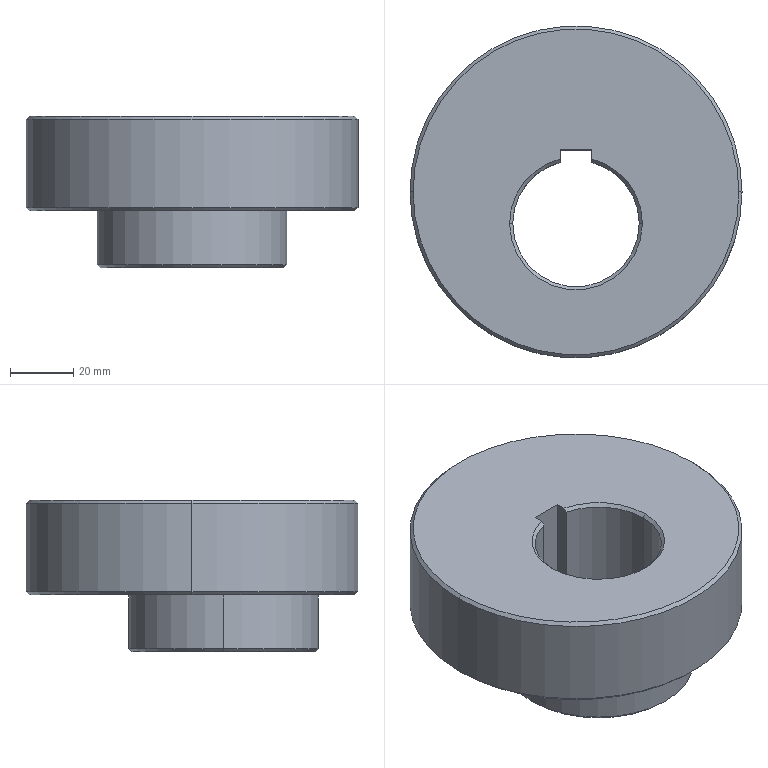Part | SolidWorks | features Boss 1, Chamfer 1, Cut 1, Extrusion 1 | 1 solid | 25 faces | box 105 x 105 x 48 mm | volume 248122 mm3 | cone 12 | cylinder 7 | plane 6 | commonest cylinder face diameters 40 x3 60 x2 105 x2
STEP:
#1=CARTESIAN_POINT('',(20.,0.,-17.));
#2=VERTEX_POINT('',#1);
#3=CARTESIAN_POINT('',(-20.,0.,-17.));
#4=VERTEX_POINT('',#3);
#5=CARTESIAN_POINT('',(0.,0.,-17.));
#6=DIRECTION('',(0.,0.,-1.));
#7=DIRECTION('',(1.,0.,0.));
#8=AXIS2_PLACEMENT_3D('',#5,#6,#7);
#9=CIRCLE('',#8,20.);
#10=EDGE_CURVE('',#2,#4,#9,.T.);
#11=ORIENTED_EDGE('',*,*,#10,.F.);
#12=CARTESIAN_POINT('',(21.,0.,-18.));
#13=VERTEX_POINT('',#12);
#14=CARTESIAN_POINT('',(21.,0.,-18.));
#15=DIRECTION('',(0.7071,0.,-0.7071));
#16=VECTOR('',#15,1000.);
#17=LINE('',#14,#16);
#18=EDGE_CURVE('',#2,#13,#17,.T.);
#19=ORIENTED_EDGE('',*,*,#18,.T.);
#20=CARTESIAN_POINT('',(-21.,0.,-18.));
#21=VERTEX_POINT('',#20);
#22=CARTESIAN_POINT('',(0.,0.,-18.));
#23=DIRECTION('',(0.,0.,1.));
#24=DIRECTION('',(1.,0.,0.));
#25=AXIS2_PLACEMENT_3D('',#22,#23,#24);
#26=CIRCLE('',#25,21.);
#27=EDGE_CURVE('',#21,#13,#26,.T.);
#28=ORIENTED_EDGE('',*,*,#27,.F.);
#29=CARTESIAN_POINT('',(-21.,0.,-18.));
#30=DIRECTION('',(-0.7071,0.,-0.7071));
#31=VECTOR('',#30,1000.);
#32=LINE('',#29,#31);
#33=EDGE_CURVE('',#4,#21,#32,.T.);
#34=ORIENTED_EDGE('',*,*,#33,.F.);
#35=EDGE_LOOP('',(#11,#19,#28,#34));
#36=FACE_OUTER_BOUND('',#35,.T.);
#37=CARTESIAN_POINT('',(0.,0.,-18.));
#38=DIRECTION('',(0.,0.,-1.));
#39=DIRECTION('',(-1.,0.,0.));
#40=AXIS2_PLACEMENT_3D('',#37,#38,#39);
#41=CONICAL_SURFACE('',#40,21.,0.7854);
#42=ADVANCED_FACE('',(#36),#41,.F.);
#43=CARTESIAN_POINT('',(-5.,19.365,-17.));
#44=VERTEX_POINT('',#43);
#45=CARTESIAN_POINT('',(0.,0.,-17.));
#46=DIRECTION('',(0.,0.,-1.));
#47=DIRECTION('',(1.,0.,0.));
#48=AXIS2_PLACEMENT_3D('',#45,#46,#47);
#49=CIRCLE('',#48,20.);
#50=EDGE_CURVE('',#4,#44,#49,.T.);
#51=ORIENTED_EDGE('',*,*,#50,.F.);
#52=ORIENTED_EDGE('',*,*,#33,.T.);
#53=CARTESIAN_POINT('',(-5.,20.396,-18.));
#54=VERTEX_POINT('',#53);
#55=CARTESIAN_POINT('',(0.,0.,-18.));
#56=DIRECTION('',(0.,0.,1.));
#57=DIRECTION('',(1.,0.,0.));
#58=AXIS2_PLACEMENT_3D('',#55,#56,#57);
#59=CIRCLE('',#58,21.);
#60=EDGE_CURVE('',#54,#21,#59,.T.);
#61=ORIENTED_EDGE('',*,*,#60,.F.);
#62=CARTESIAN_POINT('',(-5.,19.365,-17.));
#63=CARTESIAN_POINT('',(-5.,19.709,-17.333));
#64=CARTESIAN_POINT('',(-5.,20.053,-17.666));
#65=CARTESIAN_POINT('',(-5.,20.396,-18.));
#66=B_SPLINE_CURVE_WITH_KNOTS('',3,(#62,#63,#64,#65),.UNSPECIFIED.,.F.,.F.,(4,4),(0.,0.001436),.UNSPECIFIED.);
#67=EDGE_CURVE('',#44,#54,#66,.T.);
#68=ORIENTED_EDGE('',*,*,#67,.F.);
#69=EDGE_LOOP('',(#51,#52,#61,#68));
#70=FACE_OUTER_BOUND('',#69,.T.);
#71=CARTESIAN_POINT('',(0.,0.,-18.));
#72=DIRECTION('',(0.,0.,-1.));
#73=DIRECTION('',(-1.,0.,0.));
#74=AXIS2_PLACEMENT_3D('',#71,#72,#73);
#75=CONICAL_SURFACE('',#74,21.,0.7854);
#76=ADVANCED_FACE('',(#70),#75,.F.);
#77=CARTESIAN_POINT('',(-20.,0.,29.));
#78=VERTEX_POINT('',#77);
#79=CARTESIAN_POINT('',(20.,0.,29.));
#80=VERTEX_POINT('',#79);
#81=CARTESIAN_POINT('',(0.,0.,29.));
#82=DIRECTION('',(0.,0.,1.));
#83=DIRECTION('',(1.,0.,0.));
#84=AXIS2_PLACEMENT_3D('',#81,#82,#83);
#85=CIRCLE('',#84,20.);
#86=EDGE_CURVE('',#78,#80,#85,.T.);
#87=ORIENTED_EDGE('',*,*,#86,.F.);
#88=CARTESIAN_POINT('',(-21.,0.,30.));
#89=VERTEX_POINT('',#88);
#90=CARTESIAN_POINT('',(-20.,0.,29.));
#91=DIRECTION('',(-0.7071,0.,0.7071));
#92=VECTOR('',#91,1000.);
#93=LINE('',#90,#92);
#94=EDGE_CURVE('',#78,#89,#93,.T.);
#95=ORIENTED_EDGE('',*,*,#94,.T.);
#96=CARTESIAN_POINT('',(21.,0.,30.));
#97=VERTEX_POINT('',#96);
#98=CARTESIAN_POINT('',(0.,0.,30.));
#99=DIRECTION('',(0.,0.,-1.));
#100=DIRECTION('',(1.,0.,0.));
#101=AXIS2_PLACEMENT_3D('',#98,#99,#100);
#102=CIRCLE('',#101,21.);
#103=EDGE_CURVE('',#97,#89,#102,.T.);
#104=ORIENTED_EDGE('',*,*,#103,.F.);
#105=CARTESIAN_POINT('',(20.,0.,29.));
#106=DIRECTION('',(0.7071,0.,0.7071));
#107=VECTOR('',#106,1000.);
#108=LINE('',#105,#107);
#109=EDGE_CURVE('',#80,#97,#108,.T.);
#110=ORIENTED_EDGE('',*,*,#109,.F.);
#111=EDGE_LOOP('',(#87,#95,#104,#110));
#112=FACE_OUTER_BOUND('',#111,.T.);
#113=CARTESIAN_POINT('',(0.,0.,29.));
#114=DIRECTION('',(0.,0.,1.));
#115=DIRECTION('',(1.,0.,0.));
#116=AXIS2_PLACEMENT_3D('',#113,#114,#115);
#117=CONICAL_SURFACE('',#116,20.,0.7854);
#118=ADVANCED_FACE('',(#112),#117,.F.);
#119=CARTESIAN_POINT('',(5.,19.365,29.));
#120=VERTEX_POINT('',#119);
#121=CARTESIAN_POINT('',(0.,0.,29.));
#122=DIRECTION('',(0.,0.,1.));
#123=DIRECTION('',(1.,0.,0.));
#124=AXIS2_PLACEMENT_3D('',#121,#122,#123);
#125=CIRCLE('',#124,20.);
#126=EDGE_CURVE('',#80,#120,#125,.T.);
#127=ORIENTED_EDGE('',*,*,#126,.F.);
#128=ORIENTED_EDGE('',*,*,#109,.T.);
#129=CARTESIAN_POINT('',(5.,20.396,30.));
#130=VERTEX_POINT('',#129);
#131=CARTESIAN_POINT('',(0.,0.,30.));
#132=DIRECTION('',(0.,0.,-1.));
#133=DIRECTION('',(1.,0.,0.));
#134=AXIS2_PLACEMENT_3D('',#131,#132,#133);
#135=CIRCLE('',#134,21.);
#136=EDGE_CURVE('',#130,#97,#135,.T.);
#137=ORIENTED_EDGE('',*,*,#136,.F.);
#138=CARTESIAN_POINT('',(5.,19.365,29.));
#139=CARTESIAN_POINT('',(5.,19.709,29.333));
#140=CARTESIAN_POINT('',(5.,20.053,29.666));
#141=CARTESIAN_POINT('',(5.,20.396,30.));
#142=B_SPLINE_CURVE_WITH_KNOTS('',3,(#138,#139,#140,#141),.UNSPECIFIED.,.F.,.F.,(4,4),(0.,0.001436),.UNSPECIFIED.);
#143=EDGE_CURVE('',#120,#130,#142,.T.);
#144=ORIENTED_EDGE('',*,*,#143,.F.);
#145=EDGE_LOOP('',(#127,#128,#137,#144));
#146=FACE_OUTER_BOUND('',#145,.T.);
#147=CARTESIAN_POINT('',(0.,0.,29.));
#148=DIRECTION('',(0.,0.,1.));
#149=DIRECTION('',(1.,0.,0.));
#150=AXIS2_PLACEMENT_3D('',#147,#148,#149);
#151=CONICAL_SURFACE('',#150,20.,0.7854);
#152=ADVANCED_FACE('',(#146),#151,.F.);
#153=CARTESIAN_POINT('',(-29.,0.,-18.));
#154=VERTEX_POINT('',#153);
#155=CARTESIAN_POINT('',(29.,0.,-18.));
#156=VERTEX_POINT('',#155);
#157=CARTESIAN_POINT('',(0.,0.,-18.));
#158=DIRECTION('',(0.,0.,-1.));
#159=DIRECTION('',(1.,0.,0.));
#160=AXIS2_PLACEMENT_3D('',#157,#158,#159);
#161=CIRCLE('',#160,29.);
#162=EDGE_CURVE('',#154,#156,#161,.T.);
#163=ORIENTED_EDGE('',*,*,#162,.F.);
#164=CARTESIAN_POINT('',(-30.,0.,-17.));
#165=VERTEX_POINT('',#164);
#166=CARTESIAN_POINT('',(-30.,0.,-17.));
#167=DIRECTION('',(-0.7071,0.,0.7071));
#168=VECTOR('',#167,1000.);
#169=LINE('',#166,#168);
#170=EDGE_CURVE('',#154,#165,#169,.T.);
#171=ORIENTED_EDGE('',*,*,#170,.T.);
#172=CARTESIAN_POINT('',(30.,0.,-17.));
#173=VERTEX_POINT('',#172);
#174=CARTESIAN_POINT('',(0.,0.,-17.));
#175=DIRECTION('',(0.,0.,1.));
#176=DIRECTION('',(1.,0.,0.));
#177=AXIS2_PLACEMENT_3D('',#174,#175,#176);
#178=CIRCLE('',#177,30.);
#179=EDGE_CURVE('',#173,#165,#178,.T.);
#180=ORIENTED_EDGE('',*,*,#179,.F.);
#181=CARTESIAN_POINT('',(30.,0.,-17.));
#182=DIRECTION('',(0.7071,0.,0.7071));
#183=VECTOR('',#182,1000.);
#184=LINE('',#181,#183);
#185=EDGE_CURVE('',#156,#173,#184,.T.);
#186=ORIENTED_EDGE('',*,*,#185,.F.);
#187=EDGE_LOOP('',(#163,#171,#180,#186));
#188=FACE_OUTER_BOUND('',#187,.T.);
#189=CARTESIAN_POINT('',(0.,0.,-17.));
#190=DIRECTION('',(0.,0.,1.));
#191=DIRECTION('',(1.,0.,0.));
#192=AXIS2_PLACEMENT_3D('',#189,#190,#191);
#193=CONICAL_SURFACE('',#192,30.,0.7854);
#194=ADVANCED_FACE('',(#188),#193,.T.);
#195=CARTESIAN_POINT('',(-51.5,10.,0.));
#196=VERTEX_POINT('',#195);
#197=CARTESIAN_POINT('',(51.5,10.,0.));
#198=VERTEX_POINT('',#197);
#199=CARTESIAN_POINT('',(0.,10.,0.));
#200=DIRECTION('',(0.,0.,-1.));
#201=DIRECTION('',(1.,0.,0.));
#202=AXIS2_PLACEMENT_3D('',#199,#200,#201);
#203=CIRCLE('',#202,51.5);
#204=EDGE_CURVE('',#196,#198,#203,.T.);
#205=ORIENTED_EDGE('',*,*,#204,.F.);
#206=CARTESIAN_POINT('',(-52.5,10.,1.));
#207=VERTEX_POINT('',#206);
#208=CARTESIAN_POINT('',(-52.5,10.,1.));
#209=DIRECTION('',(-0.7071,0.,0.7071));
#210=VECTOR('',#209,1000.);
#211=LINE('',#208,#210);
#212=EDGE_CURVE('',#196,#207,#211,.T.);
#213=ORIENTED_EDGE('',*,*,#212,.T.);
#214=CARTESIAN_POINT('',(52.5,10.,1.));
#215=VERTEX_POINT('',#214);
#216=CARTESIAN_POINT('',(0.,10.,1.));
#217=DIRECTION('',(0.,0.,1.));
#218=DIRECTION('',(1.,0.,0.));
#219=AXIS2_PLACEMENT_3D('',#216,#217,#218);
#220=CIRCLE('',#219,52.5);
#221=EDGE_CURVE('',#215,#207,#220,.T.);
#222=ORIENTED_EDGE('',*,*,#221,.F.);
#223=CARTESIAN_POINT('',(52.5,10.,1.));
#224=DIRECTION('',(0.7071,0.,0.7071));
#225=VECTOR('',#224,1000.);
#226=LINE('',#223,#225);
#227=EDGE_CURVE('',#198,#215,#226,.T.);
#228=ORIENTED_EDGE('',*,*,#227,.F.);
#229=EDGE_LOOP('',(#205,#213,#222,#228));
#230=FACE_OUTER_BOUND('',#229,.T.);
#231=CARTESIAN_POINT('',(0.,10.,1.));
#232=DIRECTION('',(0.,0.,1.));
#233=DIRECTION('',(1.,0.,0.));
#234=AXIS2_PLACEMENT_3D('',#231,#232,#233);
#235=CONICAL_SURFACE('',#234,52.5,0.7854);
#236=ADVANCED_FACE('',(#230),#235,.T.);
#237=CARTESIAN_POINT('',(51.5,10.,30.));
#238=VERTEX_POINT('',#237);
#239=CARTESIAN_POINT('',(-51.5,10.,30.));
#240=VERTEX_POINT('',#239);
#241=CARTESIAN_POINT('',(0.,10.,30.));
#242=DIRECTION('',(0.,0.,1.));
#243=DIRECTION('',(1.,0.,0.));
#244=AXIS2_PLACEMENT_3D('',#241,#242,#243);
#245=CIRCLE('',#244,51.5);
#246=EDGE_CURVE('',#238,#240,#245,.T.);
#247=ORIENTED_EDGE('',*,*,#246,.F.);
#248=CARTESIAN_POINT('',(52.5,10.,29.));
#249=VERTEX_POINT('',#248);
#250=CARTESIAN_POINT('',(51.5,10.,30.));
#251=DIRECTION('',(0.7071,0.,-0.7071));
#252=VECTOR('',#251,1000.);
#253=LINE('',#250,#252);
#254=EDGE_CURVE('',#238,#249,#253,.T.);
#255=ORIENTED_EDGE('',*,*,#254,.T.);
#256=CARTESIAN_POINT('',(-52.5,10.,29.));
#257=VERTEX_POINT('',#256);
#258=CARTESIAN_POINT('',(0.,10.,29.));
#259=DIRECTION('',(0.,0.,-1.));
#260=DIRECTION('',(1.,0.,0.));
#261=AXIS2_PLACEMENT_3D('',#258,#259,#260);
#262=CIRCLE('',#261,52.5);
#263=EDGE_CURVE('',#257,#249,#262,.T.);
#264=ORIENTED_EDGE('',*,*,#263,.F.);
#265=CARTESIAN_POINT('',(-51.5,10.,30.));
#266=DIRECTION('',(-0.7071,0.,-0.7071));
#267=VECTOR('',#266,1000.);
#268=LINE('',#265,#267);
#269=EDGE_CURVE('',#240,#257,#268,.T.);
#270=ORIENTED_EDGE('',*,*,#269,.F.);
#271=EDGE_LOOP('',(#247,#255,#264,#270));
#272=FACE_OUTER_BOUND('',#271,.T.);
#273=CARTESIAN_POINT('',(0.,10.,30.));
#274=DIRECTION('',(0.,0.,-1.));
#275=DIRECTION('',(-1.,0.,0.));
#276=AXIS2_PLACEMENT_3D('',#273,#274,#275);
#277=CONICAL_SURFACE('',#276,51.5,0.7854);
#278=ADVANCED_FACE('',(#272),#277,.T.);
#279=ORIENTED_EDGE('',*,*,#10,.T.);
#280=CARTESIAN_POINT('',(-20.,0.,-18.));
#281=DIRECTION('',(0.,0.,1.));
#282=VECTOR('',#281,1000.);
#283=LINE('',#280,#282);
#284=EDGE_CURVE('',#4,#78,#283,.T.);
#285=ORIENTED_EDGE('',*,*,#284,.T.);
#286=ORIENTED_EDGE('',*,*,#86,.T.);
#287=CARTESIAN_POINT('',(20.,0.,-18.));
#288=DIRECTION('',(0.,0.,1.));
#289=VECTOR('',#288,1000.);
#290=LINE('',#287,#289);
#291=EDGE_CURVE('',#2,#80,#290,.T.);
#292=ORIENTED_EDGE('',*,*,#291,.F.);
#293=EDGE_LOOP('',(#279,#285,#286,#292));
#294=FACE_OUTER_BOUND('',#293,.T.);
#295=CARTESIAN_POINT('',(0.,0.,-18.));
#296=DIRECTION('',(0.,0.,1.));
#297=DIRECTION('',(1.,0.,0.));
#298=AXIS2_PLACEMENT_3D('',#295,#296,#297);
#299=CYLINDRICAL_SURFACE('',#298,20.);
#300=ADVANCED_FACE('',(#294),#299,.F.);
#301=CARTESIAN_POINT('',(5.,19.365,-17.));
#302=VERTEX_POINT('',#301);
#303=CARTESIAN_POINT('',(0.,0.,-17.));
#304=DIRECTION('',(0.,0.,-1.));
#305=DIRECTION('',(1.,0.,0.));
#306=AXIS2_PLACEMENT_3D('',#303,#304,#305);
#307=CIRCLE('',#306,20.);
#308=EDGE_CURVE('',#302,#2,#307,.T.);
#309=ORIENTED_EDGE('',*,*,#308,.T.);
#310=ORIENTED_EDGE('',*,*,#291,.T.);
#311=ORIENTED_EDGE('',*,*,#126,.T.);
#312=CARTESIAN_POINT('',(5.,19.365,-18.));
#313=DIRECTION('',(0.,0.,1.));
#314=VECTOR('',#313,1000.);
#315=LINE('',#312,#314);
#316=EDGE_CURVE('',#302,#120,#315,.T.);
#317=ORIENTED_EDGE('',*,*,#316,.F.);
#318=EDGE_LOOP('',(#309,#310,#311,#317));
#319=FACE_OUTER_BOUND('',#318,.T.);
#320=CARTESIAN_POINT('',(0.,0.,-18.));
#321=DIRECTION('',(0.,0.,1.));
#322=DIRECTION('',(1.,0.,0.));
#323=AXIS2_PLACEMENT_3D('',#320,#321,#322);
#324=CYLINDRICAL_SURFACE('',#323,20.);
#325=ADVANCED_FACE('',(#319),#324,.F.);
#326=ORIENTED_EDGE('',*,*,#179,.T.);
#327=CARTESIAN_POINT('',(-30.,0.,0.));
#328=VERTEX_POINT('',#327);
#329=CARTESIAN_POINT('',(-30.,0.,-18.));
#330=DIRECTION('',(0.,0.,1.));
#331=VECTOR('',#330,1000.);
#332=LINE('',#329,#331);
#333=EDGE_CURVE('',#165,#328,#332,.T.);
#334=ORIENTED_EDGE('',*,*,#333,.T.);
#335=CARTESIAN_POINT('',(30.,0.,0.));
#336=VERTEX_POINT('',#335);
#337=CARTESIAN_POINT('',(0.,0.,0.));
#338=DIRECTION('',(0.,0.,1.));
#339=DIRECTION('',(1.,0.,0.));
#340=AXIS2_PLACEMENT_3D('',#337,#338,#339);
#341=CIRCLE('',#340,30.);
#342=EDGE_CURVE('',#336,#328,#341,.T.);
#343=ORIENTED_EDGE('',*,*,#342,.F.);
#344=CARTESIAN_POINT('',(30.,0.,-18.));
#345=DIRECTION('',(0.,0.,1.));
#346=VECTOR('',#345,1000.);
#347=LINE('',#344,#346);
#348=EDGE_CURVE('',#173,#336,#347,.T.);
#349=ORIENTED_EDGE('',*,*,#348,.F.);
#350=EDGE_LOOP('',(#326,#334,#343,#349));
#351=FACE_OUTER_BOUND('',#350,.T.);
#352=CARTESIAN_POINT('',(0.,0.,-18.));
#353=DIRECTION('',(0.,0.,1.));
#354=DIRECTION('',(1.,0.,0.));
#355=AXIS2_PLACEMENT_3D('',#352,#353,#354);
#356=CYLINDRICAL_SURFACE('',#355,30.);
#357=ADVANCED_FACE('',(#351),#356,.T.);
#358=ORIENTED_EDGE('',*,*,#263,.T.);
#359=CARTESIAN_POINT('',(52.5,10.,30.));
#360=DIRECTION('',(0.,0.,-1.));
#361=VECTOR('',#360,1000.);
#362=LINE('',#359,#361);
#363=EDGE_CURVE('',#249,#215,#362,.T.);
#364=ORIENTED_EDGE('',*,*,#363,.T.);
#365=ORIENTED_EDGE('',*,*,#221,.T.);
#366=CARTESIAN_POINT('',(-52.5,10.,30.));
#367=DIRECTION('',(0.,0.,-1.));
#368=VECTOR('',#367,1000.);
#369=LINE('',#366,#368);
#370=EDGE_CURVE('',#257,#207,#369,.T.);
#371=ORIENTED_EDGE('',*,*,#370,.F.);
#372=EDGE_LOOP('',(#358,#364,#365,#371));
#373=FACE_OUTER_BOUND('',#372,.T.);
#374=CARTESIAN_POINT('',(0.,10.,30.));
#375=DIRECTION('',(0.,0.,-1.));
#376=DIRECTION('',(-1.,0.,0.));
#377=AXIS2_PLACEMENT_3D('',#374,#375,#376);
#378=CYLINDRICAL_SURFACE('',#377,52.5);
#379=ADVANCED_FACE('',(#373),#378,.T.);
#380=CARTESIAN_POINT('',(0.,10.,30.));
#381=DIRECTION('',(0.,0.,1.));
#382=DIRECTION('',(1.,0.,0.));
#383=AXIS2_PLACEMENT_3D('',#380,#381,#382);
#384=CIRCLE('',#383,51.5);
#385=EDGE_CURVE('',#240,#238,#384,.T.);
#386=ORIENTED_EDGE('',*,*,#385,.T.);
#387=ORIENTED_EDGE('',*,*,#246,.T.);
#388=EDGE_LOOP('',(#386,#387));
#389=FACE_OUTER_BOUND('',#388,.T.);
#390=CARTESIAN_POINT('',(5.,23.3,30.));
#391=VERTEX_POINT('',#390);
#392=CARTESIAN_POINT('',(5.,19.365,30.));
#393=DIRECTION('',(0.,1.,0.));
#394=VECTOR('',#393,1000.);
#395=LINE('',#392,#394);
#396=EDGE_CURVE('',#130,#391,#395,.T.);
#397=ORIENTED_EDGE('',*,*,#396,.F.);
#398=ORIENTED_EDGE('',*,*,#136,.T.);
#399=ORIENTED_EDGE('',*,*,#103,.T.);
#400=CARTESIAN_POINT('',(-5.,20.396,30.));
#401=VERTEX_POINT('',#400);
#402=CARTESIAN_POINT('',(0.,0.,30.));
#403=DIRECTION('',(0.,0.,-1.));
#404=DIRECTION('',(1.,0.,0.));
#405=AXIS2_PLACEMENT_3D('',#402,#403,#404);
#406=CIRCLE('',#405,21.);
#407=EDGE_CURVE('',#89,#401,#406,.T.);
#408=ORIENTED_EDGE('',*,*,#407,.T.);
#409=CARTESIAN_POINT('',(-5.,23.3,30.));
#410=VERTEX_POINT('',#409);
#411=CARTESIAN_POINT('',(-5.,23.3,30.));
#412=DIRECTION('',(0.,-1.,0.));
#413=VECTOR('',#412,1000.);
#414=LINE('',#411,#413);
#415=EDGE_CURVE('',#410,#401,#414,.T.);
#416=ORIENTED_EDGE('',*,*,#415,.F.);
#417=CARTESIAN_POINT('',(5.,23.3,30.));
#418=DIRECTION('',(-1.,0.,0.));
#419=VECTOR('',#418,1000.);
#420=LINE('',#417,#419);
#421=EDGE_CURVE('',#391,#410,#420,.T.);
#422=ORIENTED_EDGE('',*,*,#421,.F.);
#423=EDGE_LOOP('',(#397,#398,#399,#408,#416,#422));
#424=FACE_BOUND('',#423,.T.);
#425=CARTESIAN_POINT('',(0.,10.,30.));
#426=DIRECTION('',(0.,0.,1.));
#427=DIRECTION('',(1.,0.,0.));
#428=AXIS2_PLACEMENT_3D('',#425,#426,#427);
#429=PLANE('',#428);
#430=ADVANCED_FACE('',(#389,#424),#429,.T.);
#431=ORIENTED_EDGE('',*,*,#363,.F.);
#432=CARTESIAN_POINT('',(0.,10.,29.));
#433=DIRECTION('',(0.,0.,-1.));
#434=DIRECTION('',(1.,0.,0.));
#435=AXIS2_PLACEMENT_3D('',#432,#433,#434);
#436=CIRCLE('',#435,52.5);
#437=EDGE_CURVE('',#249,#257,#436,.T.);
#438=ORIENTED_EDGE('',*,*,#437,.T.);
#439=ORIENTED_EDGE('',*,*,#370,.T.);
#440=CARTESIAN_POINT('',(0.,10.,1.));
#441=DIRECTION('',(0.,0.,1.));
#442=DIRECTION('',(1.,0.,0.));
#443=AXIS2_PLACEMENT_3D('',#440,#441,#442);
#444=CIRCLE('',#443,52.5);
#445=EDGE_CURVE('',#207,#215,#444,.T.);
#446=ORIENTED_EDGE('',*,*,#445,.T.);
#447=EDGE_LOOP('',(#431,#438,#439,#446));
#448=FACE_OUTER_BOUND('',#447,.T.);
#449=CARTESIAN_POINT('',(0.,10.,30.));
#450=DIRECTION('',(0.,0.,-1.));
#451=DIRECTION('',(-1.,0.,0.));
#452=AXIS2_PLACEMENT_3D('',#449,#450,#451);
#453=CYLINDRICAL_SURFACE('',#452,52.5);
#454=ADVANCED_FACE('',(#448),#453,.T.);
#455=CARTESIAN_POINT('',(0.,10.,0.));
#456=DIRECTION('',(0.,0.,-1.));
#457=DIRECTION('',(1.,0.,0.));
#458=AXIS2_PLACEMENT_3D('',#455,#456,#457);
#459=CIRCLE('',#458,51.5);
#460=EDGE_CURVE('',#198,#196,#459,.T.);
#461=ORIENTED_EDGE('',*,*,#460,.T.);
#462=ORIENTED_EDGE('',*,*,#204,.T.);
#463=EDGE_LOOP('',(#461,#462));
#464=FACE_OUTER_BOUND('',#463,.T.);
#465=ORIENTED_EDGE('',*,*,#342,.T.);
#466=CARTESIAN_POINT('',(0.,0.,0.));
#467=DIRECTION('',(0.,0.,1.));
#468=DIRECTION('',(1.,0.,0.));
#469=AXIS2_PLACEMENT_3D('',#466,#467,#468);
#470=CIRCLE('',#469,30.);
#471=EDGE_CURVE('',#328,#336,#470,.T.);
#472=ORIENTED_EDGE('',*,*,#471,.T.);
#473=EDGE_LOOP('',(#465,#472));
#474=FACE_BOUND('',#473,.T.);
#475=CARTESIAN_POINT('',(0.,10.,0.));
#476=DIRECTION('',(0.,0.,1.));
#477=DIRECTION('',(1.,0.,0.));
#478=AXIS2_PLACEMENT_3D('',#475,#476,#477);
#479=PLANE('',#478);
#480=ADVANCED_FACE('',(#464,#474),#479,.F.);
#481=ORIENTED_EDGE('',*,*,#333,.F.);
#482=CARTESIAN_POINT('',(0.,0.,-17.));
#483=DIRECTION('',(0.,0.,1.));
#484=DIRECTION('',(1.,0.,0.));
#485=AXIS2_PLACEMENT_3D('',#482,#483,#484);
#486=CIRCLE('',#485,30.);
#487=EDGE_CURVE('',#165,#173,#486,.T.);
#488=ORIENTED_EDGE('',*,*,#487,.T.);
#489=ORIENTED_EDGE('',*,*,#348,.T.);
#490=ORIENTED_EDGE('',*,*,#471,.F.);
#491=EDGE_LOOP('',(#481,#488,#489,#490));
#492=FACE_OUTER_BOUND('',#491,.T.);
#493=CARTESIAN_POINT('',(0.,0.,-18.));
#494=DIRECTION('',(0.,0.,1.));
#495=DIRECTION('',(1.,0.,0.));
#496=AXIS2_PLACEMENT_3D('',#493,#494,#495);
#497=CYLINDRICAL_SURFACE('',#496,30.);
#498=ADVANCED_FACE('',(#492),#497,.T.);
#499=CARTESIAN_POINT('',(0.,0.,-18.));
#500=DIRECTION('',(0.,0.,-1.));
#501=DIRECTION('',(1.,0.,0.));
#502=AXIS2_PLACEMENT_3D('',#499,#500,#501);
#503=CIRCLE('',#502,29.);
#504=EDGE_CURVE('',#156,#154,#503,.T.);
#505=ORIENTED_EDGE('',*,*,#504,.T.);
#506=ORIENTED_EDGE('',*,*,#162,.T.);
#507=EDGE_LOOP('',(#505,#506));
#508=FACE_OUTER_BOUND('',#507,.T.);
#509=CARTESIAN_POINT('',(-5.,23.3,-18.));
#510=VERTEX_POINT('',#509);
#511=CARTESIAN_POINT('',(-5.,23.3,-18.));
#512=DIRECTION('',(0.,-1.,0.));
#513=VECTOR('',#512,1000.);
#514=LINE('',#511,#513);
#515=EDGE_CURVE('',#510,#54,#514,.T.);
#516=ORIENTED_EDGE('',*,*,#515,.T.);
#517=ORIENTED_EDGE('',*,*,#60,.T.);
#518=ORIENTED_EDGE('',*,*,#27,.T.);
#519=CARTESIAN_POINT('',(5.,20.396,-18.));
#520=VERTEX_POINT('',#519);
#521=CARTESIAN_POINT('',(0.,0.,-18.));
#522=DIRECTION('',(0.,0.,1.));
#523=DIRECTION('',(1.,0.,0.));
#524=AXIS2_PLACEMENT_3D('',#521,#522,#523);
#525=CIRCLE('',#524,21.);
#526=EDGE_CURVE('',#13,#520,#525,.T.);
#527=ORIENTED_EDGE('',*,*,#526,.T.);
#528=CARTESIAN_POINT('',(5.,23.3,-18.));
#529=VERTEX_POINT('',#528);
#530=CARTESIAN_POINT('',(5.,19.365,-18.));
#531=DIRECTION('',(0.,1.,0.));
#532=VECTOR('',#531,1000.);
#533=LINE('',#530,#532);
#534=EDGE_CURVE('',#520,#529,#533,.T.);
#535=ORIENTED_EDGE('',*,*,#534,.T.);
#536=CARTESIAN_POINT('',(5.,23.3,-18.));
#537=DIRECTION('',(-1.,0.,0.));
#538=VECTOR('',#537,1000.);
#539=LINE('',#536,#538);
#540=EDGE_CURVE('',#529,#510,#539,.T.);
#541=ORIENTED_EDGE('',*,*,#540,.T.);
#542=EDGE_LOOP('',(#516,#517,#518,#527,#535,#541));
#543=FACE_BOUND('',#542,.T.);
#544=CARTESIAN_POINT('',(0.,0.,-18.));
#545=DIRECTION('',(0.,0.,1.));
#546=DIRECTION('',(1.,0.,0.));
#547=AXIS2_PLACEMENT_3D('',#544,#545,#546);
#548=PLANE('',#547);
#549=ADVANCED_FACE('',(#508,#543),#548,.F.);
#550=ORIENTED_EDGE('',*,*,#415,.T.);
#551=CARTESIAN_POINT('',(-5.,19.365,29.));
#552=VERTEX_POINT('',#551);
#553=CARTESIAN_POINT('',(-5.,20.396,30.));
#554=CARTESIAN_POINT('',(-5.,20.053,29.666));
#555=CARTESIAN_POINT('',(-5.,19.709,29.333));
#556=CARTESIAN_POINT('',(-5.,19.365,29.));
#557=B_SPLINE_CURVE_WITH_KNOTS('',3,(#553,#554,#555,#556),.UNSPECIFIED.,.F.,.F.,(4,4),(0.,0.001436),.UNSPECIFIED.);
#558=EDGE_CURVE('',#401,#552,#557,.T.);
#559=ORIENTED_EDGE('',*,*,#558,.T.);
#560=CARTESIAN_POINT('',(-5.,19.365,-18.));
#561=DIRECTION('',(0.,0.,1.));
#562=VECTOR('',#561,1000.);
#563=LINE('',#560,#562);
#564=EDGE_CURVE('',#44,#552,#563,.T.);
#565=ORIENTED_EDGE('',*,*,#564,.F.);
#566=ORIENTED_EDGE('',*,*,#67,.T.);
#567=ORIENTED_EDGE('',*,*,#515,.F.);
#568=CARTESIAN_POINT('',(-5.,23.3,-18.));
#569=DIRECTION('',(0.,0.,1.));
#570=VECTOR('',#569,1000.);
#571=LINE('',#568,#570);
#572=EDGE_CURVE('',#510,#410,#571,.T.);
#573=ORIENTED_EDGE('',*,*,#572,.T.);
#574=EDGE_LOOP('',(#550,#559,#565,#566,#567,#573));
#575=FACE_OUTER_BOUND('',#574,.T.);
#576=CARTESIAN_POINT('',(-5.,23.3,-18.));
#577=DIRECTION('',(-1.,0.,0.));
#578=DIRECTION('',(0.,-1.,0.));
#579=AXIS2_PLACEMENT_3D('',#576,#577,#578);
#580=PLANE('',#579);
#581=ADVANCED_FACE('',(#575),#580,.F.);
#582=CARTESIAN_POINT('',(5.,23.3,-18.));
#583=DIRECTION('',(0.,0.,1.));
#584=VECTOR('',#583,1000.);
#585=LINE('',#582,#584);
#586=EDGE_CURVE('',#529,#391,#585,.T.);
#587=ORIENTED_EDGE('',*,*,#586,.T.);
#588=ORIENTED_EDGE('',*,*,#421,.T.);
#589=ORIENTED_EDGE('',*,*,#572,.F.);
#590=ORIENTED_EDGE('',*,*,#540,.F.);
#591=EDGE_LOOP('',(#587,#588,#589,#590));
#592=FACE_OUTER_BOUND('',#591,.T.);
#593=CARTESIAN_POINT('',(5.,23.3,-18.));
#594=DIRECTION('',(0.,1.,0.));
#595=DIRECTION('',(0.,0.,1.));
#596=AXIS2_PLACEMENT_3D('',#593,#594,#595);
#597=PLANE('',#596);
#598=ADVANCED_FACE('',(#592),#597,.F.);
#599=ORIENTED_EDGE('',*,*,#316,.T.);
#600=ORIENTED_EDGE('',*,*,#143,.T.);
#601=ORIENTED_EDGE('',*,*,#396,.T.);
#602=ORIENTED_EDGE('',*,*,#586,.F.);
#603=ORIENTED_EDGE('',*,*,#534,.F.);
#604=CARTESIAN_POINT('',(5.,20.396,-18.));
#605=CARTESIAN_POINT('',(5.,20.053,-17.666));
#606=CARTESIAN_POINT('',(5.,19.709,-17.333));
#607=CARTESIAN_POINT('',(5.,19.365,-17.));
#608=B_SPLINE_CURVE_WITH_KNOTS('',3,(#604,#605,#606,#607),.UNSPECIFIED.,.F.,.F.,(4,4),(0.,0.001436),.UNSPECIFIED.);
#609=EDGE_CURVE('',#520,#302,#608,.T.);
#610=ORIENTED_EDGE('',*,*,#609,.T.);
#611=EDGE_LOOP('',(#599,#600,#601,#602,#603,#610));
#612=FACE_OUTER_BOUND('',#611,.T.);
#613=CARTESIAN_POINT('',(5.,19.365,-18.));
#614=DIRECTION('',(1.,0.,0.));
#615=DIRECTION('',(0.,1.,0.));
#616=AXIS2_PLACEMENT_3D('',#613,#614,#615);
#617=PLANE('',#616);
#618=ADVANCED_FACE('',(#612),#617,.F.);
#619=ORIENTED_EDGE('',*,*,#284,.F.);
#620=ORIENTED_EDGE('',*,*,#50,.T.);
#621=ORIENTED_EDGE('',*,*,#564,.T.);
#622=CARTESIAN_POINT('',(0.,0.,29.));
#623=DIRECTION('',(0.,0.,1.));
#624=DIRECTION('',(1.,0.,0.));
#625=AXIS2_PLACEMENT_3D('',#622,#623,#624);
#626=CIRCLE('',#625,20.);
#627=EDGE_CURVE('',#552,#78,#626,.T.);
#628=ORIENTED_EDGE('',*,*,#627,.T.);
#629=EDGE_LOOP('',(#619,#620,#621,#628));
#630=FACE_OUTER_BOUND('',#629,.T.);
#631=CARTESIAN_POINT('',(0.,0.,-18.));
#632=DIRECTION('',(0.,0.,1.));
#633=DIRECTION('',(1.,0.,0.));
#634=AXIS2_PLACEMENT_3D('',#631,#632,#633);
#635=CYLINDRICAL_SURFACE('',#634,20.);
#636=ADVANCED_FACE('',(#630),#635,.F.);
#637=ORIENTED_EDGE('',*,*,#254,.F.);
#638=ORIENTED_EDGE('',*,*,#385,.F.);
#639=ORIENTED_EDGE('',*,*,#269,.T.);
#640=ORIENTED_EDGE('',*,*,#437,.F.);
#641=EDGE_LOOP('',(#637,#638,#639,#640));
#642=FACE_OUTER_BOUND('',#641,.T.);
#643=CARTESIAN_POINT('',(0.,10.,30.));
#644=DIRECTION('',(0.,0.,-1.));
#645=DIRECTION('',(-1.,0.,0.));
#646=AXIS2_PLACEMENT_3D('',#643,#644,#645);
#647=CONICAL_SURFACE('',#646,51.5,0.7854);
#648=ADVANCED_FACE('',(#642),#647,.T.);
#649=ORIENTED_EDGE('',*,*,#212,.F.);
#650=ORIENTED_EDGE('',*,*,#460,.F.);
#651=ORIENTED_EDGE('',*,*,#227,.T.);
#652=ORIENTED_EDGE('',*,*,#445,.F.);
#653=EDGE_LOOP('',(#649,#650,#651,#652));
#654=FACE_OUTER_BOUND('',#653,.T.);
#655=CARTESIAN_POINT('',(0.,10.,1.));
#656=DIRECTION('',(0.,0.,1.));
#657=DIRECTION('',(1.,0.,0.));
#658=AXIS2_PLACEMENT_3D('',#655,#656,#657);
#659=CONICAL_SURFACE('',#658,52.5,0.7854);
#660=ADVANCED_FACE('',(#654),#659,.T.);
#661=ORIENTED_EDGE('',*,*,#170,.F.);
#662=ORIENTED_EDGE('',*,*,#504,.F.);
#663=ORIENTED_EDGE('',*,*,#185,.T.);
#664=ORIENTED_EDGE('',*,*,#487,.F.);
#665=EDGE_LOOP('',(#661,#662,#663,#664));
#666=FACE_OUTER_BOUND('',#665,.T.);
#667=CARTESIAN_POINT('',(0.,0.,-17.));
#668=DIRECTION('',(0.,0.,1.));
#669=DIRECTION('',(1.,0.,0.));
#670=AXIS2_PLACEMENT_3D('',#667,#668,#669);
#671=CONICAL_SURFACE('',#670,30.,0.7854);
#672=ADVANCED_FACE('',(#666),#671,.T.);
#673=ORIENTED_EDGE('',*,*,#94,.F.);
#674=ORIENTED_EDGE('',*,*,#627,.F.);
#675=ORIENTED_EDGE('',*,*,#558,.F.);
#676=ORIENTED_EDGE('',*,*,#407,.F.);
#677=EDGE_LOOP('',(#673,#674,#675,#676));
#678=FACE_OUTER_BOUND('',#677,.T.);
#679=CARTESIAN_POINT('',(0.,0.,29.));
#680=DIRECTION('',(0.,0.,1.));
#681=DIRECTION('',(1.,0.,0.));
#682=AXIS2_PLACEMENT_3D('',#679,#680,#681);
#683=CONICAL_SURFACE('',#682,20.,0.7854);
#684=ADVANCED_FACE('',(#678),#683,.F.);
#685=ORIENTED_EDGE('',*,*,#18,.F.);
#686=ORIENTED_EDGE('',*,*,#308,.F.);
#687=ORIENTED_EDGE('',*,*,#609,.F.);
#688=ORIENTED_EDGE('',*,*,#526,.F.);
#689=EDGE_LOOP('',(#685,#686,#687,#688));
#690=FACE_OUTER_BOUND('',#689,.T.);
#691=CARTESIAN_POINT('',(0.,0.,-18.));
#692=DIRECTION('',(0.,0.,-1.));
#693=DIRECTION('',(-1.,0.,0.));
#694=AXIS2_PLACEMENT_3D('',#691,#692,#693);
#695=CONICAL_SURFACE('',#694,21.,0.7854);
#696=ADVANCED_FACE('',(#690),#695,.F.);
#697=CLOSED_SHELL('',(#42,#76,#118,#152,#194,#236,#278,#300,#325,#357,#379,#430,#454,#480,#498,#549,#581,#598,#618,#636,#648,#660,#672,#684,#696));
#698=MANIFOLD_SOLID_BREP('',#697);
#699=CARTESIAN_POINT('',(0.,0.,0.));
#700=DIRECTION('',(0.,0.,1.));
#701=DIRECTION('',(1.,0.,0.));
#702=AXIS2_PLACEMENT_3D('',#699,#700,#701);
#703=(LENGTH_UNIT()NAMED_UNIT(*)SI_UNIT(.MILLI.,.METRE.));
#704=UNCERTAINTY_MEASURE_WITH_UNIT(LENGTH_MEASURE(0.00001),#703,'','');
#705=(NAMED_UNIT(*)PLANE_ANGLE_UNIT()SI_UNIT($,.RADIAN.));
#706=(NAMED_UNIT(*)SI_UNIT($,.STERADIAN.)SOLID_ANGLE_UNIT());
#707=(GEOMETRIC_REPRESENTATION_CONTEXT(3)GLOBAL_UNCERTAINTY_ASSIGNED_CONTEXT((#704))GLOBAL_UNIT_ASSIGNED_CONTEXT((#703,#705,#706))REPRESENTATION_CONTEXT('',''));
#708=ADVANCED_BREP_SHAPE_REPRESENTATION('',(#698,#702),#707);